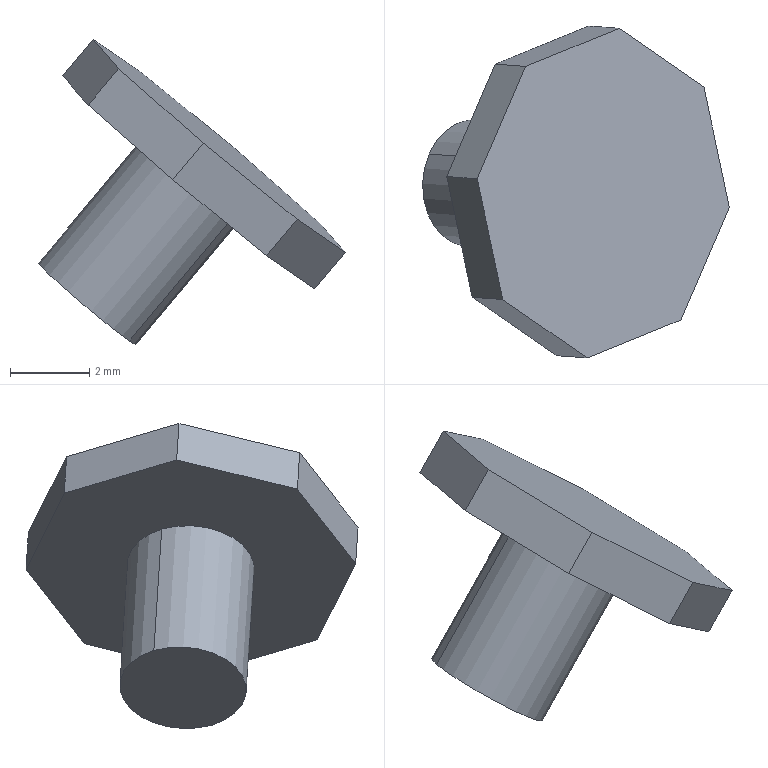Part | SolidWorks | features SplitBody 1 | 1 solid | 13 faces | box 7.745 x 8.38 x 7.699 mm | volume 91.502 mm3 | plane 11 | cylinder 2 | commonest cylinder face diameters 3.2 x2
STEP:
#1=CARTESIAN_POINT('',(526.049,311.35,-337.758));
#2=VERTEX_POINT('',#1);
#3=CARTESIAN_POINT('',(528.181,309.878,-339.638));
#4=VERTEX_POINT('',#3);
#5=CARTESIAN_POINT('',(527.115,310.614,-338.698));
#6=DIRECTION('',(-0.6411,0.04931,-0.7658));
#7=DIRECTION('',(-0.6661,0.4599,0.5872));
#8=AXIS2_PLACEMENT_3D('',#5,#6,#7);
#9=CIRCLE('',#8,1.6);
#10=EDGE_CURVE('',#2,#4,#9,.T.);
#11=ORIENTED_EDGE('',*,*,#10,.F.);
#12=CARTESIAN_POINT('',(528.614,311.152,-334.695));
#13=VERTEX_POINT('',#12);
#14=CARTESIAN_POINT('',(526.049,311.35,-337.758));
#15=DIRECTION('',(0.6411,-0.04931,0.7658));
#16=VECTOR('',#15,1000.);
#17=LINE('',#14,#16);
#18=EDGE_CURVE('',#2,#13,#17,.T.);
#19=ORIENTED_EDGE('',*,*,#18,.T.);
#20=CARTESIAN_POINT('',(530.745,309.681,-336.574));
#21=VERTEX_POINT('',#20);
#22=CARTESIAN_POINT('',(529.679,310.417,-335.635));
#23=DIRECTION('',(-0.6411,0.04931,-0.7658));
#24=DIRECTION('',(-0.6661,0.4599,0.5872));
#25=AXIS2_PLACEMENT_3D('',#22,#23,#24);
#26=CIRCLE('',#25,1.6);
#27=EDGE_CURVE('',#13,#21,#26,.T.);
#28=ORIENTED_EDGE('',*,*,#27,.T.);
#29=CARTESIAN_POINT('',(528.181,309.878,-339.638));
#30=DIRECTION('',(0.6411,-0.04931,0.7658));
#31=VECTOR('',#30,1000.);
#32=LINE('',#29,#31);
#33=EDGE_CURVE('',#4,#21,#32,.T.);
#34=ORIENTED_EDGE('',*,*,#33,.F.);
#35=EDGE_LOOP('',(#11,#19,#28,#34));
#36=FACE_OUTER_BOUND('',#35,.T.);
#37=CARTESIAN_POINT('',(527.115,310.614,-338.698));
#38=DIRECTION('',(0.6411,-0.04931,0.7658));
#39=DIRECTION('',(0.6661,-0.4599,-0.5872));
#40=AXIS2_PLACEMENT_3D('',#37,#38,#39);
#41=CYLINDRICAL_SURFACE('',#40,1.6);
#42=ADVANCED_FACE('',(#36),#41,.T.);
#43=CARTESIAN_POINT('',(527.911,307.669,-332.764));
#44=VERTEX_POINT('',#43);
#45=CARTESIAN_POINT('',(527.266,310.715,-332.028));
#46=VERTEX_POINT('',#45);
#47=CARTESIAN_POINT('',(527.911,307.669,-332.764));
#48=DIRECTION('',(-0.2015,0.9521,0.23));
#49=VECTOR('',#48,1000.);
#50=LINE('',#47,#49);
#51=EDGE_CURVE('',#44,#46,#50,.T.);
#52=ORIENTED_EDGE('',*,*,#51,.T.);
#53=CARTESIAN_POINT('',(526.497,310.775,-332.947));
#54=VERTEX_POINT('',#53);
#55=CARTESIAN_POINT('',(526.497,310.775,-332.947));
#56=DIRECTION('',(0.6411,-0.04931,0.7658));
#57=VECTOR('',#56,1000.);
#58=LINE('',#55,#57);
#59=EDGE_CURVE('',#54,#46,#58,.T.);
#60=ORIENTED_EDGE('',*,*,#59,.F.);
#61=CARTESIAN_POINT('',(527.141,307.728,-333.683));
#62=VERTEX_POINT('',#61);
#63=CARTESIAN_POINT('',(527.141,307.728,-333.683));
#64=DIRECTION('',(-0.2015,0.9521,0.23));
#65=VECTOR('',#64,1000.);
#66=LINE('',#63,#65);
#67=EDGE_CURVE('',#62,#54,#66,.T.);
#68=ORIENTED_EDGE('',*,*,#67,.F.);
#69=CARTESIAN_POINT('',(527.141,307.728,-333.683));
#70=DIRECTION('',(0.6411,-0.04931,0.7658));
#71=VECTOR('',#70,1000.);
#72=LINE('',#69,#71);
#73=EDGE_CURVE('',#62,#44,#72,.T.);
#74=ORIENTED_EDGE('',*,*,#73,.T.);
#75=EDGE_LOOP('',(#52,#60,#68,#74));
#76=FACE_OUTER_BOUND('',#75,.T.);
#77=CARTESIAN_POINT('',(527.141,307.728,-333.683));
#78=DIRECTION('',(0.7405,0.3017,-0.6005));
#79=DIRECTION('',(0.2015,-0.9521,-0.23));
#80=AXIS2_PLACEMENT_3D('',#77,#78,#79);
#81=PLANE('',#80);
#82=ADVANCED_FACE('',(#76),#81,.F.);
#83=CARTESIAN_POINT('',(528.486,313.552,-332.867));
#84=VERTEX_POINT('',#83);
#85=CARTESIAN_POINT('',(527.266,310.715,-332.028));
#86=DIRECTION('',(0.3812,0.8866,-0.262));
#87=VECTOR('',#86,1000.);
#88=LINE('',#85,#87);
#89=EDGE_CURVE('',#46,#84,#88,.T.);
#90=ORIENTED_EDGE('',*,*,#89,.T.);
#91=CARTESIAN_POINT('',(527.716,313.612,-333.786));
#92=VERTEX_POINT('',#91);
#93=CARTESIAN_POINT('',(527.716,313.612,-333.786));
#94=DIRECTION('',(0.6411,-0.04931,0.7658));
#95=VECTOR('',#94,1000.);
#96=LINE('',#93,#95);
#97=EDGE_CURVE('',#92,#84,#96,.T.);
#98=ORIENTED_EDGE('',*,*,#97,.F.);
#99=CARTESIAN_POINT('',(526.497,310.775,-332.947));
#100=DIRECTION('',(0.3812,0.8866,-0.262));
#101=VECTOR('',#100,1000.);
#102=LINE('',#99,#101);
#103=EDGE_CURVE('',#54,#92,#102,.T.);
#104=ORIENTED_EDGE('',*,*,#103,.F.);
#105=ORIENTED_EDGE('',*,*,#59,.T.);
#106=EDGE_LOOP('',(#90,#98,#104,#105));
#107=FACE_OUTER_BOUND('',#106,.T.);
#108=CARTESIAN_POINT('',(526.497,310.775,-332.947));
#109=DIRECTION('',(0.6661,-0.4599,-0.5872));
#110=DIRECTION('',(-0.3812,-0.8866,0.262));
#111=AXIS2_PLACEMENT_3D('',#108,#109,#110);
#112=PLANE('',#111);
#113=ADVANCED_FACE('',(#107),#112,.F.);
#114=CARTESIAN_POINT('',(530.855,314.518,-334.788));
#115=VERTEX_POINT('',#114);
#116=CARTESIAN_POINT('',(528.486,313.552,-332.867));
#117=DIRECTION('',(0.7405,0.3017,-0.6005));
#118=VECTOR('',#117,1000.);
#119=LINE('',#116,#118);
#120=EDGE_CURVE('',#84,#115,#119,.T.);
#121=ORIENTED_EDGE('',*,*,#120,.T.);
#122=CARTESIAN_POINT('',(530.086,314.577,-335.707));
#123=VERTEX_POINT('',#122);
#124=CARTESIAN_POINT('',(530.086,314.577,-335.707));
#125=DIRECTION('',(0.6411,-0.04931,0.7658));
#126=VECTOR('',#125,1000.);
#127=LINE('',#124,#126);
#128=EDGE_CURVE('',#123,#115,#127,.T.);
#129=ORIENTED_EDGE('',*,*,#128,.F.);
#130=CARTESIAN_POINT('',(527.716,313.612,-333.786));
#131=DIRECTION('',(0.7405,0.3017,-0.6005));
#132=VECTOR('',#131,1000.);
#133=LINE('',#130,#132);
#134=EDGE_CURVE('',#92,#123,#133,.T.);
#135=ORIENTED_EDGE('',*,*,#134,.F.);
#136=ORIENTED_EDGE('',*,*,#97,.T.);
#137=EDGE_LOOP('',(#121,#129,#135,#136));
#138=FACE_OUTER_BOUND('',#137,.T.);
#139=CARTESIAN_POINT('',(527.716,313.612,-333.786));
#140=DIRECTION('',(0.2015,-0.9521,-0.23));
#141=DIRECTION('',(-0.7405,-0.3017,0.6005));
#142=AXIS2_PLACEMENT_3D('',#139,#140,#141);
#143=PLANE('',#142);
#144=ADVANCED_FACE('',(#138),#143,.F.);
#145=CARTESIAN_POINT('',(532.987,313.046,-336.667));
#146=VERTEX_POINT('',#145);
#147=CARTESIAN_POINT('',(530.855,314.518,-334.788));
#148=DIRECTION('',(0.6661,-0.4599,-0.5872));
#149=VECTOR('',#148,1000.);
#150=LINE('',#147,#149);
#151=EDGE_CURVE('',#115,#146,#150,.T.);
#152=ORIENTED_EDGE('',*,*,#151,.T.);
#153=CARTESIAN_POINT('',(532.217,313.106,-337.586));
#154=VERTEX_POINT('',#153);
#155=CARTESIAN_POINT('',(532.217,313.106,-337.586));
#156=DIRECTION('',(0.6411,-0.04931,0.7658));
#157=VECTOR('',#156,1000.);
#158=LINE('',#155,#157);
#159=EDGE_CURVE('',#154,#146,#158,.T.);
#160=ORIENTED_EDGE('',*,*,#159,.F.);
#161=CARTESIAN_POINT('',(530.086,314.577,-335.707));
#162=DIRECTION('',(0.6661,-0.4599,-0.5872));
#163=VECTOR('',#162,1000.);
#164=LINE('',#161,#163);
#165=EDGE_CURVE('',#123,#154,#164,.T.);
#166=ORIENTED_EDGE('',*,*,#165,.F.);
#167=ORIENTED_EDGE('',*,*,#128,.T.);
#168=EDGE_LOOP('',(#152,#160,#166,#167));
#169=FACE_OUTER_BOUND('',#168,.T.);
#170=CARTESIAN_POINT('',(530.086,314.577,-335.707));
#171=DIRECTION('',(-0.3812,-0.8866,0.262));
#172=DIRECTION('',(-0.6661,0.4599,0.5872));
#173=AXIS2_PLACEMENT_3D('',#170,#171,#172);
#174=PLANE('',#173);
#175=ADVANCED_FACE('',(#169),#174,.F.);
#176=CARTESIAN_POINT('',(533.632,310.,-337.403));
#177=VERTEX_POINT('',#176);
#178=CARTESIAN_POINT('',(532.987,313.046,-336.667));
#179=DIRECTION('',(0.2015,-0.9521,-0.23));
#180=VECTOR('',#179,1000.);
#181=LINE('',#178,#180);
#182=EDGE_CURVE('',#146,#177,#181,.T.);
#183=ORIENTED_EDGE('',*,*,#182,.T.);
#184=CARTESIAN_POINT('',(532.862,310.059,-338.322));
#185=VERTEX_POINT('',#184);
#186=CARTESIAN_POINT('',(532.862,310.059,-338.322));
#187=DIRECTION('',(0.6411,-0.04931,0.7658));
#188=VECTOR('',#187,1000.);
#189=LINE('',#186,#188);
#190=EDGE_CURVE('',#185,#177,#189,.T.);
#191=ORIENTED_EDGE('',*,*,#190,.F.);
#192=CARTESIAN_POINT('',(532.217,313.106,-337.586));
#193=DIRECTION('',(0.2015,-0.9521,-0.23));
#194=VECTOR('',#193,1000.);
#195=LINE('',#192,#194);
#196=EDGE_CURVE('',#154,#185,#195,.T.);
#197=ORIENTED_EDGE('',*,*,#196,.F.);
#198=ORIENTED_EDGE('',*,*,#159,.T.);
#199=EDGE_LOOP('',(#183,#191,#197,#198));
#200=FACE_OUTER_BOUND('',#199,.T.);
#201=CARTESIAN_POINT('',(532.217,313.106,-337.586));
#202=DIRECTION('',(-0.7405,-0.3017,0.6005));
#203=DIRECTION('',(-0.2015,0.9521,0.23));
#204=AXIS2_PLACEMENT_3D('',#201,#202,#203);
#205=PLANE('',#204);
#206=ADVANCED_FACE('',(#200),#205,.F.);
#207=CARTESIAN_POINT('',(532.412,307.163,-336.565));
#208=VERTEX_POINT('',#207);
#209=CARTESIAN_POINT('',(533.632,310.,-337.403));
#210=DIRECTION('',(-0.3812,-0.8866,0.262));
#211=VECTOR('',#210,1000.);
#212=LINE('',#209,#211);
#213=EDGE_CURVE('',#177,#208,#212,.T.);
#214=ORIENTED_EDGE('',*,*,#213,.T.);
#215=CARTESIAN_POINT('',(531.642,307.222,-337.484));
#216=VERTEX_POINT('',#215);
#217=CARTESIAN_POINT('',(531.642,307.222,-337.484));
#218=DIRECTION('',(0.6411,-0.04931,0.7658));
#219=VECTOR('',#218,1000.);
#220=LINE('',#217,#219);
#221=EDGE_CURVE('',#216,#208,#220,.T.);
#222=ORIENTED_EDGE('',*,*,#221,.F.);
#223=CARTESIAN_POINT('',(532.862,310.059,-338.322));
#224=DIRECTION('',(-0.3812,-0.8866,0.262));
#225=VECTOR('',#224,1000.);
#226=LINE('',#223,#225);
#227=EDGE_CURVE('',#185,#216,#226,.T.);
#228=ORIENTED_EDGE('',*,*,#227,.F.);
#229=ORIENTED_EDGE('',*,*,#190,.T.);
#230=EDGE_LOOP('',(#214,#222,#228,#229));
#231=FACE_OUTER_BOUND('',#230,.T.);
#232=CARTESIAN_POINT('',(532.862,310.059,-338.322));
#233=DIRECTION('',(-0.6661,0.4599,0.5872));
#234=DIRECTION('',(0.3812,0.8866,-0.262));
#235=AXIS2_PLACEMENT_3D('',#232,#233,#234);
#236=PLANE('',#235);
#237=ADVANCED_FACE('',(#231),#236,.F.);
#238=CARTESIAN_POINT('',(530.042,306.197,-334.643));
#239=VERTEX_POINT('',#238);
#240=CARTESIAN_POINT('',(532.412,307.163,-336.565));
#241=DIRECTION('',(-0.7405,-0.3017,0.6005));
#242=VECTOR('',#241,1000.);
#243=LINE('',#240,#242);
#244=EDGE_CURVE('',#208,#239,#243,.T.);
#245=ORIENTED_EDGE('',*,*,#244,.T.);
#246=CARTESIAN_POINT('',(529.273,306.256,-335.562));
#247=VERTEX_POINT('',#246);
#248=CARTESIAN_POINT('',(529.273,306.256,-335.562));
#249=DIRECTION('',(0.6411,-0.04931,0.7658));
#250=VECTOR('',#249,1000.);
#251=LINE('',#248,#250);
#252=EDGE_CURVE('',#247,#239,#251,.T.);
#253=ORIENTED_EDGE('',*,*,#252,.F.);
#254=CARTESIAN_POINT('',(531.642,307.222,-337.484));
#255=DIRECTION('',(-0.7405,-0.3017,0.6005));
#256=VECTOR('',#255,1000.);
#257=LINE('',#254,#256);
#258=EDGE_CURVE('',#216,#247,#257,.T.);
#259=ORIENTED_EDGE('',*,*,#258,.F.);
#260=ORIENTED_EDGE('',*,*,#221,.T.);
#261=EDGE_LOOP('',(#245,#253,#259,#260));
#262=FACE_OUTER_BOUND('',#261,.T.);
#263=CARTESIAN_POINT('',(531.642,307.222,-337.484));
#264=DIRECTION('',(-0.2015,0.9521,0.23));
#265=DIRECTION('',(0.7405,0.3017,-0.6005));
#266=AXIS2_PLACEMENT_3D('',#263,#264,#265);
#267=PLANE('',#266);
#268=ADVANCED_FACE('',(#262),#267,.F.);
#269=CARTESIAN_POINT('',(530.042,306.197,-334.643));
#270=DIRECTION('',(-0.6661,0.4599,0.5872));
#271=VECTOR('',#270,1000.);
#272=LINE('',#269,#271);
#273=EDGE_CURVE('',#239,#44,#272,.T.);
#274=ORIENTED_EDGE('',*,*,#273,.T.);
#275=ORIENTED_EDGE('',*,*,#73,.F.);
#276=CARTESIAN_POINT('',(529.273,306.256,-335.562));
#277=DIRECTION('',(-0.6661,0.4599,0.5872));
#278=VECTOR('',#277,1000.);
#279=LINE('',#276,#278);
#280=EDGE_CURVE('',#247,#62,#279,.T.);
#281=ORIENTED_EDGE('',*,*,#280,.F.);
#282=ORIENTED_EDGE('',*,*,#252,.T.);
#283=EDGE_LOOP('',(#274,#275,#281,#282));
#284=FACE_OUTER_BOUND('',#283,.T.);
#285=CARTESIAN_POINT('',(529.273,306.256,-335.562));
#286=DIRECTION('',(0.3812,0.8866,-0.262));
#287=DIRECTION('',(0.6661,-0.4599,-0.5872));
#288=AXIS2_PLACEMENT_3D('',#285,#286,#287);
#289=PLANE('',#288);
#290=ADVANCED_FACE('',(#284),#289,.F.);
#291=CARTESIAN_POINT('',(529.679,310.417,-335.635));
#292=DIRECTION('',(-0.6411,0.04931,-0.7658));
#293=DIRECTION('',(-0.6661,0.4599,0.5872));
#294=AXIS2_PLACEMENT_3D('',#291,#292,#293);
#295=CIRCLE('',#294,1.6);
#296=EDGE_CURVE('',#21,#13,#295,.T.);
#297=ORIENTED_EDGE('',*,*,#296,.F.);
#298=ORIENTED_EDGE('',*,*,#27,.F.);
#299=EDGE_LOOP('',(#297,#298));
#300=FACE_BOUND('',#299,.T.);
#301=ORIENTED_EDGE('',*,*,#67,.T.);
#302=ORIENTED_EDGE('',*,*,#103,.T.);
#303=ORIENTED_EDGE('',*,*,#134,.T.);
#304=ORIENTED_EDGE('',*,*,#165,.T.);
#305=ORIENTED_EDGE('',*,*,#196,.T.);
#306=ORIENTED_EDGE('',*,*,#227,.T.);
#307=ORIENTED_EDGE('',*,*,#258,.T.);
#308=ORIENTED_EDGE('',*,*,#280,.T.);
#309=EDGE_LOOP('',(#301,#302,#303,#304,#305,#306,#307,#308));
#310=FACE_OUTER_BOUND('',#309,.T.);
#311=CARTESIAN_POINT('',(529.679,310.417,-335.635));
#312=DIRECTION('',(-0.6411,0.04931,-0.7658));
#313=DIRECTION('',(-0.6661,0.4599,0.5872));
#314=AXIS2_PLACEMENT_3D('',#311,#312,#313);
#315=PLANE('',#314);
#316=ADVANCED_FACE('',(#300,#310),#315,.T.);
#317=ORIENTED_EDGE('',*,*,#51,.F.);
#318=ORIENTED_EDGE('',*,*,#273,.F.);
#319=ORIENTED_EDGE('',*,*,#244,.F.);
#320=ORIENTED_EDGE('',*,*,#213,.F.);
#321=ORIENTED_EDGE('',*,*,#182,.F.);
#322=ORIENTED_EDGE('',*,*,#151,.F.);
#323=ORIENTED_EDGE('',*,*,#120,.F.);
#324=ORIENTED_EDGE('',*,*,#89,.F.);
#325=EDGE_LOOP('',(#317,#318,#319,#320,#321,#322,#323,#324));
#326=FACE_OUTER_BOUND('',#325,.T.);
#327=CARTESIAN_POINT('',(530.449,310.358,-334.716));
#328=DIRECTION('',(-0.6411,0.04931,-0.7658));
#329=DIRECTION('',(-0.6661,0.4599,0.5872));
#330=AXIS2_PLACEMENT_3D('',#327,#328,#329);
#331=PLANE('',#330);
#332=ADVANCED_FACE('',(#326),#331,.F.);
#333=ORIENTED_EDGE('',*,*,#18,.F.);
#334=CARTESIAN_POINT('',(527.115,310.614,-338.698));
#335=DIRECTION('',(-0.6411,0.04931,-0.7658));
#336=DIRECTION('',(-0.6661,0.4599,0.5872));
#337=AXIS2_PLACEMENT_3D('',#334,#335,#336);
#338=CIRCLE('',#337,1.6);
#339=EDGE_CURVE('',#4,#2,#338,.T.);
#340=ORIENTED_EDGE('',*,*,#339,.F.);
#341=ORIENTED_EDGE('',*,*,#33,.T.);
#342=ORIENTED_EDGE('',*,*,#296,.T.);
#343=EDGE_LOOP('',(#333,#340,#341,#342));
#344=FACE_OUTER_BOUND('',#343,.T.);
#345=CARTESIAN_POINT('',(527.115,310.614,-338.698));
#346=DIRECTION('',(0.6411,-0.04931,0.7658));
#347=DIRECTION('',(0.6661,-0.4599,-0.5872));
#348=AXIS2_PLACEMENT_3D('',#345,#346,#347);
#349=CYLINDRICAL_SURFACE('',#348,1.6);
#350=ADVANCED_FACE('',(#344),#349,.T.);
#351=ORIENTED_EDGE('',*,*,#339,.T.);
#352=ORIENTED_EDGE('',*,*,#10,.T.);
#353=EDGE_LOOP('',(#351,#352));
#354=FACE_OUTER_BOUND('',#353,.T.);
#355=CARTESIAN_POINT('',(527.115,310.614,-338.698));
#356=DIRECTION('',(-0.6411,0.04931,-0.7658));
#357=DIRECTION('',(-0.6661,0.4599,0.5872));
#358=AXIS2_PLACEMENT_3D('',#355,#356,#357);
#359=PLANE('',#358);
#360=ADVANCED_FACE('',(#354),#359,.T.);
#361=CLOSED_SHELL('',(#42,#82,#113,#144,#175,#206,#237,#268,#290,#316,#332,#350,#360));
#362=MANIFOLD_SOLID_BREP('',#361);
#363=CARTESIAN_POINT('',(0.,0.,0.));
#364=DIRECTION('',(0.,0.,1.));
#365=DIRECTION('',(1.,0.,0.));
#366=AXIS2_PLACEMENT_3D('',#363,#364,#365);
#367=(LENGTH_UNIT()NAMED_UNIT(*)SI_UNIT(.MILLI.,.METRE.));
#368=UNCERTAINTY_MEASURE_WITH_UNIT(LENGTH_MEASURE(0.00001),#367,'','');
#369=(NAMED_UNIT(*)PLANE_ANGLE_UNIT()SI_UNIT($,.RADIAN.));
#370=(NAMED_UNIT(*)SI_UNIT($,.STERADIAN.)SOLID_ANGLE_UNIT());
#371=(GEOMETRIC_REPRESENTATION_CONTEXT(3)GLOBAL_UNCERTAINTY_ASSIGNED_CONTEXT((#368))GLOBAL_UNIT_ASSIGNED_CONTEXT((#367,#369,#370))REPRESENTATION_CONTEXT('',''));
#372=ADVANCED_BREP_SHAPE_REPRESENTATION('',(#362,#366),#371);